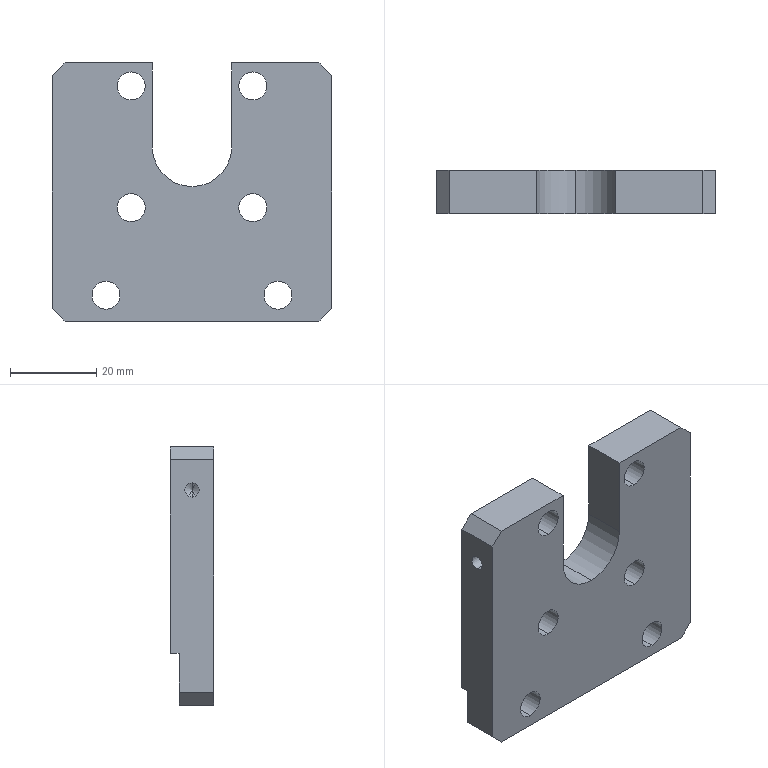Part | STEP file | PN_0007 | 1 solid | 33 faces | box 65 x 10 x 60 mm | volume 30379 mm3 | cylinder 16 | plane 15 | cone 2 | commonest cylinder face diameters 6.5 x12 3.3 x2 18.5 x2